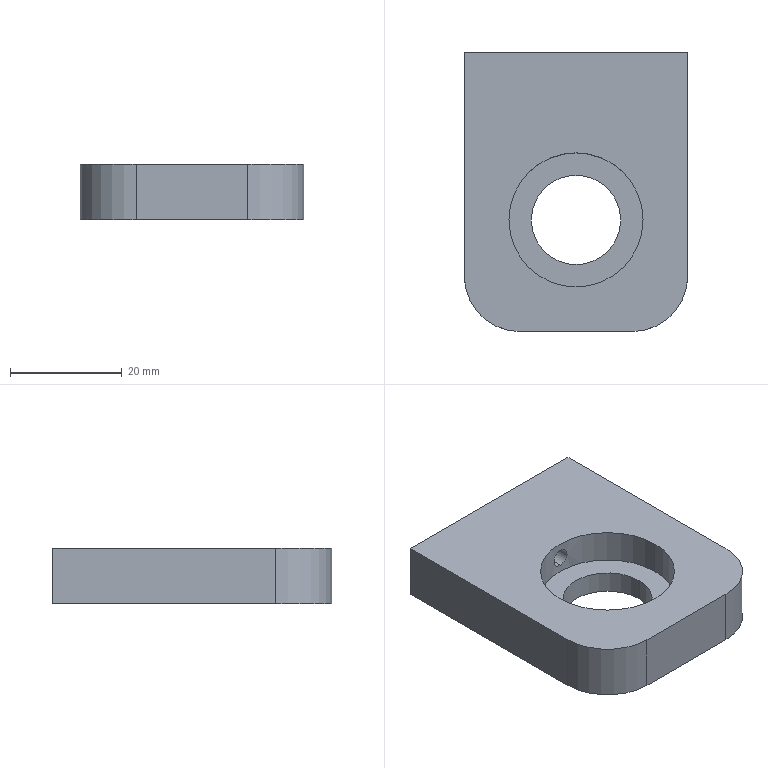Part | SolidWorks | features HoleWzd 2, ICE 2, Extrusion 1, Fillet 1 | 1 solid | 23 faces | box 40 x 50 x 10 mm | volume 15721 mm3 | cylinder 12 | plane 7 | cone 4 | commonest cylinder face diameters 3.3 x6 16 x2 20 x2 24 x2
STEP:
#1=CARTESIAN_POINT('',(0.,7.,5.35));
#2=VERTEX_POINT('',#1);
#3=CARTESIAN_POINT('',(0.,7.,8.65));
#4=VERTEX_POINT('',#3);
#5=CARTESIAN_POINT('',(0.,7.,5.35));
#6=CARTESIAN_POINT('',(-0.2155,7.,5.35));
#7=CARTESIAN_POINT('',(-0.4328,6.994,5.393));
#8=CARTESIAN_POINT('',(-0.8299,6.973,5.558));
#9=CARTESIAN_POINT('',(-1.014,6.958,5.681));
#10=CARTESIAN_POINT('',(-1.242,6.936,5.908));
#11=CARTESIAN_POINT('',(-1.312,6.928,5.993));
#12=CARTESIAN_POINT('',(-1.431,6.914,6.172));
#13=CARTESIAN_POINT('',(-1.482,6.908,6.267));
#14=CARTESIAN_POINT('',(-1.565,6.898,6.467));
#15=CARTESIAN_POINT('',(-1.597,6.893,6.571));
#16=CARTESIAN_POINT('',(-1.639,6.888,6.782));
#17=CARTESIAN_POINT('',(-1.65,6.886,6.89));
#18=CARTESIAN_POINT('',(-1.65,6.886,7.108));
#19=CARTESIAN_POINT('',(-1.639,6.888,7.215));
#20=CARTESIAN_POINT('',(-1.598,6.893,7.426));
#21=CARTESIAN_POINT('',(-1.566,6.897,7.531));
#22=CARTESIAN_POINT('',(-1.483,6.908,7.731));
#23=CARTESIAN_POINT('',(-1.433,6.914,7.826));
#24=CARTESIAN_POINT('',(-1.313,6.928,8.005));
#25=CARTESIAN_POINT('',(-1.243,6.936,8.09));
#26=CARTESIAN_POINT('',(-1.016,6.958,8.318));
#27=CARTESIAN_POINT('',(-0.8319,6.973,8.441));
#28=CARTESIAN_POINT('',(-0.4351,6.994,8.606));
#29=CARTESIAN_POINT('',(-0.2183,7.,8.65));
#30=CARTESIAN_POINT('',(0.,7.,8.65));
#31=B_SPLINE_CURVE_WITH_KNOTS('',3,(#5,#6,#7,#8,#9,#10,#11,#12,#13,#14,#15,#16,#17,#18,#19,#20,#21,#22,#23,#24,#25,#26,#27,#28,#29,#30),.UNSPECIFIED.,.F.,.F.,(4,2,2,2,2,2,2,2,2,2,2,2,4),(0.005165,0.00581,0.006456,0.006778,0.007101,0.007424,0.007747,0.008069,0.008392,0.008715,0.009037,0.009683,0.01033),.UNSPECIFIED.);
#32=EDGE_CURVE('',#2,#4,#31,.T.);
#33=ORIENTED_EDGE('',*,*,#32,.F.);
#34=CARTESIAN_POINT('',(0.,25.,5.35));
#35=VERTEX_POINT('',#34);
#36=CARTESIAN_POINT('',(0.,25.,5.35));
#37=DIRECTION('',(0.,1.,0.));
#38=VECTOR('',#37,1000.);
#39=LINE('',#36,#38);
#40=EDGE_CURVE('',#2,#35,#39,.T.);
#41=ORIENTED_EDGE('',*,*,#40,.T.);
#42=CARTESIAN_POINT('',(0.,25.,8.65));
#43=VERTEX_POINT('',#42);
#44=CARTESIAN_POINT('',(0.,25.,7.));
#45=DIRECTION('',(0.,1.,0.));
#46=DIRECTION('',(0.,0.,1.));
#47=AXIS2_PLACEMENT_3D('',#44,#45,#46);
#48=CIRCLE('',#47,1.65);
#49=EDGE_CURVE('',#35,#43,#48,.T.);
#50=ORIENTED_EDGE('',*,*,#49,.T.);
#51=CARTESIAN_POINT('',(0.,25.,8.65));
#52=DIRECTION('',(0.,1.,0.));
#53=VECTOR('',#52,1000.);
#54=LINE('',#51,#53);
#55=EDGE_CURVE('',#4,#43,#54,.T.);
#56=ORIENTED_EDGE('',*,*,#55,.F.);
#57=EDGE_LOOP('',(#33,#41,#50,#56));
#58=FACE_OUTER_BOUND('',#57,.T.);
#59=CARTESIAN_POINT('',(0.,25.,7.));
#60=DIRECTION('',(0.,1.,0.));
#61=DIRECTION('',(0.,0.,1.));
#62=AXIS2_PLACEMENT_3D('',#59,#60,#61);
#63=CYLINDRICAL_SURFACE('',#62,1.65);
#64=ADVANCED_FACE('',(#58),#63,.F.);
#65=CARTESIAN_POINT('',(-15.,15.,3.35));
#66=VERTEX_POINT('',#65);
#67=CARTESIAN_POINT('',(-15.,15.,6.65));
#68=VERTEX_POINT('',#67);
#69=CARTESIAN_POINT('',(-15.,15.,5.));
#70=DIRECTION('',(0.,1.,0.));
#71=DIRECTION('',(0.,0.,1.));
#72=AXIS2_PLACEMENT_3D('',#69,#70,#71);
#73=CIRCLE('',#72,1.65);
#74=EDGE_CURVE('',#66,#68,#73,.T.);
#75=ORIENTED_EDGE('',*,*,#74,.F.);
#76=CARTESIAN_POINT('',(-15.,25.,3.35));
#77=VERTEX_POINT('',#76);
#78=CARTESIAN_POINT('',(-15.,25.,3.35));
#79=DIRECTION('',(0.,1.,0.));
#80=VECTOR('',#79,1000.);
#81=LINE('',#78,#80);
#82=EDGE_CURVE('',#66,#77,#81,.T.);
#83=ORIENTED_EDGE('',*,*,#82,.T.);
#84=CARTESIAN_POINT('',(-15.,25.,6.65));
#85=VERTEX_POINT('',#84);
#86=CARTESIAN_POINT('',(-15.,25.,5.));
#87=DIRECTION('',(0.,1.,0.));
#88=DIRECTION('',(0.,0.,1.));
#89=AXIS2_PLACEMENT_3D('',#86,#87,#88);
#90=CIRCLE('',#89,1.65);
#91=EDGE_CURVE('',#77,#85,#90,.T.);
#92=ORIENTED_EDGE('',*,*,#91,.T.);
#93=CARTESIAN_POINT('',(-15.,25.,6.65));
#94=DIRECTION('',(0.,1.,0.));
#95=VECTOR('',#94,1000.);
#96=LINE('',#93,#95);
#97=EDGE_CURVE('',#68,#85,#96,.T.);
#98=ORIENTED_EDGE('',*,*,#97,.F.);
#99=EDGE_LOOP('',(#75,#83,#92,#98));
#100=FACE_OUTER_BOUND('',#99,.T.);
#101=CARTESIAN_POINT('',(-15.,25.,5.));
#102=DIRECTION('',(0.,1.,0.));
#103=DIRECTION('',(0.,0.,1.));
#104=AXIS2_PLACEMENT_3D('',#101,#102,#103);
#105=CYLINDRICAL_SURFACE('',#104,1.65);
#106=ADVANCED_FACE('',(#100),#105,.F.);
#107=CARTESIAN_POINT('',(-15.,14.009,5.));
#108=VERTEX_POINT('',#107);
#109=CARTESIAN_POINT('',(-15.,15.,6.65));
#110=DIRECTION('',(0.,0.515,0.8572));
#111=VECTOR('',#110,1000.);
#112=LINE('',#109,#111);
#113=EDGE_CURVE('',#108,#68,#112,.T.);
#114=ORIENTED_EDGE('',*,*,#113,.F.);
#115=CARTESIAN_POINT('',(-15.,15.,3.35));
#116=DIRECTION('',(0.,0.515,-0.8572));
#117=VECTOR('',#116,1000.);
#118=LINE('',#115,#117);
#119=EDGE_CURVE('',#108,#66,#118,.T.);
#120=ORIENTED_EDGE('',*,*,#119,.T.);
#121=ORIENTED_EDGE('',*,*,#74,.T.);
#122=EDGE_LOOP('',(#114,#120,#121));
#123=FACE_OUTER_BOUND('',#122,.T.);
#124=CARTESIAN_POINT('',(-15.,15.,5.));
#125=DIRECTION('',(0.,1.,0.));
#126=DIRECTION('',(0.,0.,1.));
#127=AXIS2_PLACEMENT_3D('',#124,#125,#126);
#128=CONICAL_SURFACE('',#127,1.65,1.03);
#129=ADVANCED_FACE('',(#123),#128,.F.);
#130=CARTESIAN_POINT('',(15.,15.,3.35));
#131=VERTEX_POINT('',#130);
#132=CARTESIAN_POINT('',(15.,15.,6.65));
#133=VERTEX_POINT('',#132);
#134=CARTESIAN_POINT('',(15.,15.,5.));
#135=DIRECTION('',(0.,1.,0.));
#136=DIRECTION('',(0.,0.,1.));
#137=AXIS2_PLACEMENT_3D('',#134,#135,#136);
#138=CIRCLE('',#137,1.65);
#139=EDGE_CURVE('',#131,#133,#138,.T.);
#140=ORIENTED_EDGE('',*,*,#139,.F.);
#141=CARTESIAN_POINT('',(15.,25.,3.35));
#142=VERTEX_POINT('',#141);
#143=CARTESIAN_POINT('',(15.,25.,3.35));
#144=DIRECTION('',(0.,1.,0.));
#145=VECTOR('',#144,1000.);
#146=LINE('',#143,#145);
#147=EDGE_CURVE('',#131,#142,#146,.T.);
#148=ORIENTED_EDGE('',*,*,#147,.T.);
#149=CARTESIAN_POINT('',(15.,25.,6.65));
#150=VERTEX_POINT('',#149);
#151=CARTESIAN_POINT('',(15.,25.,5.));
#152=DIRECTION('',(0.,1.,0.));
#153=DIRECTION('',(0.,0.,1.));
#154=AXIS2_PLACEMENT_3D('',#151,#152,#153);
#155=CIRCLE('',#154,1.65);
#156=EDGE_CURVE('',#142,#150,#155,.T.);
#157=ORIENTED_EDGE('',*,*,#156,.T.);
#158=CARTESIAN_POINT('',(15.,25.,6.65));
#159=DIRECTION('',(0.,1.,0.));
#160=VECTOR('',#159,1000.);
#161=LINE('',#158,#160);
#162=EDGE_CURVE('',#133,#150,#161,.T.);
#163=ORIENTED_EDGE('',*,*,#162,.F.);
#164=EDGE_LOOP('',(#140,#148,#157,#163));
#165=FACE_OUTER_BOUND('',#164,.T.);
#166=CARTESIAN_POINT('',(15.,25.,5.));
#167=DIRECTION('',(0.,1.,0.));
#168=DIRECTION('',(0.,0.,1.));
#169=AXIS2_PLACEMENT_3D('',#166,#167,#168);
#170=CYLINDRICAL_SURFACE('',#169,1.65);
#171=ADVANCED_FACE('',(#165),#170,.F.);
#172=CARTESIAN_POINT('',(15.,14.009,5.));
#173=VERTEX_POINT('',#172);
#174=CARTESIAN_POINT('',(15.,15.,6.65));
#175=DIRECTION('',(0.,0.515,0.8572));
#176=VECTOR('',#175,1000.);
#177=LINE('',#174,#176);
#178=EDGE_CURVE('',#173,#133,#177,.T.);
#179=ORIENTED_EDGE('',*,*,#178,.F.);
#180=CARTESIAN_POINT('',(15.,15.,3.35));
#181=DIRECTION('',(0.,0.515,-0.8572));
#182=VECTOR('',#181,1000.);
#183=LINE('',#180,#182);
#184=EDGE_CURVE('',#173,#131,#183,.T.);
#185=ORIENTED_EDGE('',*,*,#184,.T.);
#186=ORIENTED_EDGE('',*,*,#139,.T.);
#187=EDGE_LOOP('',(#179,#185,#186));
#188=FACE_OUTER_BOUND('',#187,.T.);
#189=CARTESIAN_POINT('',(15.,15.,5.));
#190=DIRECTION('',(0.,1.,0.));
#191=DIRECTION('',(0.,0.,1.));
#192=AXIS2_PLACEMENT_3D('',#189,#190,#191);
#193=CONICAL_SURFACE('',#192,1.65,1.03);
#194=ADVANCED_FACE('',(#188),#193,.F.);
#195=CARTESIAN_POINT('',(-8.,-5.,0.));
#196=VERTEX_POINT('',#195);
#197=CARTESIAN_POINT('',(8.,-5.,0.));
#198=VERTEX_POINT('',#197);
#199=CARTESIAN_POINT('',(0.,-5.,0.));
#200=DIRECTION('',(0.,0.,1.));
#201=DIRECTION('',(1.,0.,0.));
#202=AXIS2_PLACEMENT_3D('',#199,#200,#201);
#203=CIRCLE('',#202,8.);
#204=EDGE_CURVE('',#196,#198,#203,.T.);
#205=ORIENTED_EDGE('',*,*,#204,.F.);
#206=CARTESIAN_POINT('',(-8.,-5.,4.));
#207=VERTEX_POINT('',#206);
#208=CARTESIAN_POINT('',(-8.,-5.,0.));
#209=DIRECTION('',(0.,0.,1.));
#210=VECTOR('',#209,1000.);
#211=LINE('',#208,#210);
#212=EDGE_CURVE('',#196,#207,#211,.T.);
#213=ORIENTED_EDGE('',*,*,#212,.T.);
#214=CARTESIAN_POINT('',(8.,-5.,4.));
#215=VERTEX_POINT('',#214);
#216=CARTESIAN_POINT('',(0.,-5.,4.));
#217=DIRECTION('',(0.,0.,1.));
#218=DIRECTION('',(1.,0.,0.));
#219=AXIS2_PLACEMENT_3D('',#216,#217,#218);
#220=CIRCLE('',#219,8.);
#221=EDGE_CURVE('',#207,#215,#220,.T.);
#222=ORIENTED_EDGE('',*,*,#221,.T.);
#223=CARTESIAN_POINT('',(8.,-5.,0.));
#224=DIRECTION('',(0.,0.,1.));
#225=VECTOR('',#224,1000.);
#226=LINE('',#223,#225);
#227=EDGE_CURVE('',#198,#215,#226,.T.);
#228=ORIENTED_EDGE('',*,*,#227,.F.);
#229=EDGE_LOOP('',(#205,#213,#222,#228));
#230=FACE_OUTER_BOUND('',#229,.T.);
#231=CARTESIAN_POINT('',(0.,-5.,0.));
#232=DIRECTION('',(0.,0.,1.));
#233=DIRECTION('',(1.,0.,0.));
#234=AXIS2_PLACEMENT_3D('',#231,#232,#233);
#235=CYLINDRICAL_SURFACE('',#234,8.);
#236=ADVANCED_FACE('',(#230),#235,.F.);
#237=CARTESIAN_POINT('',(-12.,-5.,4.));
#238=VERTEX_POINT('',#237);
#239=CARTESIAN_POINT('',(12.,-5.,4.));
#240=VERTEX_POINT('',#239);
#241=CARTESIAN_POINT('',(0.,-5.,4.));
#242=DIRECTION('',(0.,0.,1.));
#243=DIRECTION('',(1.,0.,0.));
#244=AXIS2_PLACEMENT_3D('',#241,#242,#243);
#245=CIRCLE('',#244,12.);
#246=EDGE_CURVE('',#238,#240,#245,.T.);
#247=ORIENTED_EDGE('',*,*,#246,.F.);
#248=CARTESIAN_POINT('',(-12.,-5.,10.));
#249=VERTEX_POINT('',#248);
#250=CARTESIAN_POINT('',(-12.,-5.,4.));
#251=DIRECTION('',(0.,0.,1.));
#252=VECTOR('',#251,1000.);
#253=LINE('',#250,#252);
#254=EDGE_CURVE('',#238,#249,#253,.T.);
#255=ORIENTED_EDGE('',*,*,#254,.T.);
#256=CARTESIAN_POINT('',(12.,-5.,10.));
#257=VERTEX_POINT('',#256);
#258=CARTESIAN_POINT('',(0.,-5.,10.));
#259=DIRECTION('',(0.,0.,1.));
#260=DIRECTION('',(1.,0.,0.));
#261=AXIS2_PLACEMENT_3D('',#258,#259,#260);
#262=CIRCLE('',#261,12.);
#263=EDGE_CURVE('',#249,#257,#262,.T.);
#264=ORIENTED_EDGE('',*,*,#263,.T.);
#265=CARTESIAN_POINT('',(12.,-5.,4.));
#266=DIRECTION('',(0.,0.,1.));
#267=VECTOR('',#266,1000.);
#268=LINE('',#265,#267);
#269=EDGE_CURVE('',#240,#257,#268,.T.);
#270=ORIENTED_EDGE('',*,*,#269,.F.);
#271=EDGE_LOOP('',(#247,#255,#264,#270));
#272=FACE_OUTER_BOUND('',#271,.T.);
#273=CARTESIAN_POINT('',(0.,-5.,4.));
#274=DIRECTION('',(0.,0.,1.));
#275=DIRECTION('',(1.,0.,0.));
#276=AXIS2_PLACEMENT_3D('',#273,#274,#275);
#277=CYLINDRICAL_SURFACE('',#276,12.);
#278=ADVANCED_FACE('',(#272),#277,.F.);
#279=CARTESIAN_POINT('',(-20.,25.,0.));
#280=VERTEX_POINT('',#279);
#281=CARTESIAN_POINT('',(-20.,-15.,0.));
#282=VERTEX_POINT('',#281);
#283=CARTESIAN_POINT('',(-20.,25.,0.));
#284=DIRECTION('',(0.,-1.,0.));
#285=VECTOR('',#284,1000.);
#286=LINE('',#283,#285);
#287=EDGE_CURVE('',#280,#282,#286,.T.);
#288=ORIENTED_EDGE('',*,*,#287,.T.);
#289=CARTESIAN_POINT('',(-20.,-15.,10.));
#290=VERTEX_POINT('',#289);
#291=CARTESIAN_POINT('',(-20.,-15.,10.));
#292=DIRECTION('',(0.,0.,1.));
#293=VECTOR('',#292,1000.);
#294=LINE('',#291,#293);
#295=EDGE_CURVE('',#282,#290,#294,.T.);
#296=ORIENTED_EDGE('',*,*,#295,.T.);
#297=CARTESIAN_POINT('',(-20.,25.,10.));
#298=VERTEX_POINT('',#297);
#299=CARTESIAN_POINT('',(-20.,25.,10.));
#300=DIRECTION('',(0.,-1.,0.));
#301=VECTOR('',#300,1000.);
#302=LINE('',#299,#301);
#303=EDGE_CURVE('',#298,#290,#302,.T.);
#304=ORIENTED_EDGE('',*,*,#303,.F.);
#305=CARTESIAN_POINT('',(-20.,25.,10.));
#306=DIRECTION('',(0.,0.,-1.));
#307=VECTOR('',#306,1000.);
#308=LINE('',#305,#307);
#309=EDGE_CURVE('',#298,#280,#308,.T.);
#310=ORIENTED_EDGE('',*,*,#309,.T.);
#311=EDGE_LOOP('',(#288,#296,#304,#310));
#312=FACE_OUTER_BOUND('',#311,.T.);
#313=CARTESIAN_POINT('',(-20.,25.,10.));
#314=DIRECTION('',(1.,0.,0.));
#315=DIRECTION('',(0.,1.,0.));
#316=AXIS2_PLACEMENT_3D('',#313,#314,#315);
#317=PLANE('',#316);
#318=ADVANCED_FACE('',(#312),#317,.F.);
#319=CARTESIAN_POINT('',(-10.,-25.,10.));
#320=VERTEX_POINT('',#319);
#321=CARTESIAN_POINT('',(10.,-25.,10.));
#322=VERTEX_POINT('',#321);
#323=CARTESIAN_POINT('',(20.,-25.,10.));
#324=DIRECTION('',(1.,0.,0.));
#325=VECTOR('',#324,1000.);
#326=LINE('',#323,#325);
#327=EDGE_CURVE('',#320,#322,#326,.T.);
#328=ORIENTED_EDGE('',*,*,#327,.F.);
#329=CARTESIAN_POINT('',(-10.,-25.,0.));
#330=VERTEX_POINT('',#329);
#331=CARTESIAN_POINT('',(-10.,-25.,10.));
#332=DIRECTION('',(0.,0.,-1.));
#333=VECTOR('',#332,1000.);
#334=LINE('',#331,#333);
#335=EDGE_CURVE('',#320,#330,#334,.T.);
#336=ORIENTED_EDGE('',*,*,#335,.T.);
#337=CARTESIAN_POINT('',(10.,-25.,0.));
#338=VERTEX_POINT('',#337);
#339=CARTESIAN_POINT('',(20.,-25.,0.));
#340=DIRECTION('',(1.,0.,0.));
#341=VECTOR('',#340,1000.);
#342=LINE('',#339,#341);
#343=EDGE_CURVE('',#330,#338,#342,.T.);
#344=ORIENTED_EDGE('',*,*,#343,.T.);
#345=CARTESIAN_POINT('',(10.,-25.,10.));
#346=DIRECTION('',(0.,0.,1.));
#347=VECTOR('',#346,1000.);
#348=LINE('',#345,#347);
#349=EDGE_CURVE('',#338,#322,#348,.T.);
#350=ORIENTED_EDGE('',*,*,#349,.T.);
#351=EDGE_LOOP('',(#328,#336,#344,#350));
#352=FACE_OUTER_BOUND('',#351,.T.);
#353=CARTESIAN_POINT('',(20.,-25.,10.));
#354=DIRECTION('',(0.,1.,0.));
#355=DIRECTION('',(-1.,0.,0.));
#356=AXIS2_PLACEMENT_3D('',#353,#354,#355);
#357=PLANE('',#356);
#358=ADVANCED_FACE('',(#352),#357,.F.);
#359=CARTESIAN_POINT('',(20.,-15.,10.));
#360=VERTEX_POINT('',#359);
#361=CARTESIAN_POINT('',(20.,25.,10.));
#362=VERTEX_POINT('',#361);
#363=CARTESIAN_POINT('',(20.,25.,10.));
#364=DIRECTION('',(0.,1.,0.));
#365=VECTOR('',#364,1000.);
#366=LINE('',#363,#365);
#367=EDGE_CURVE('',#360,#362,#366,.T.);
#368=ORIENTED_EDGE('',*,*,#367,.F.);
#369=CARTESIAN_POINT('',(20.,-15.,0.));
#370=VERTEX_POINT('',#369);
#371=CARTESIAN_POINT('',(20.,-15.,10.));
#372=DIRECTION('',(0.,0.,-1.));
#373=VECTOR('',#372,1000.);
#374=LINE('',#371,#373);
#375=EDGE_CURVE('',#360,#370,#374,.T.);
#376=ORIENTED_EDGE('',*,*,#375,.T.);
#377=CARTESIAN_POINT('',(20.,25.,0.));
#378=VERTEX_POINT('',#377);
#379=CARTESIAN_POINT('',(20.,25.,0.));
#380=DIRECTION('',(0.,1.,0.));
#381=VECTOR('',#380,1000.);
#382=LINE('',#379,#381);
#383=EDGE_CURVE('',#370,#378,#382,.T.);
#384=ORIENTED_EDGE('',*,*,#383,.T.);
#385=CARTESIAN_POINT('',(20.,25.,10.));
#386=DIRECTION('',(0.,0.,-1.));
#387=VECTOR('',#386,1000.);
#388=LINE('',#385,#387);
#389=EDGE_CURVE('',#362,#378,#388,.T.);
#390=ORIENTED_EDGE('',*,*,#389,.F.);
#391=EDGE_LOOP('',(#368,#376,#384,#390));
#392=FACE_OUTER_BOUND('',#391,.T.);
#393=CARTESIAN_POINT('',(20.,25.,10.));
#394=DIRECTION('',(-1.,0.,0.));
#395=DIRECTION('',(0.,-1.,0.));
#396=AXIS2_PLACEMENT_3D('',#393,#394,#395);
#397=PLANE('',#396);
#398=ADVANCED_FACE('',(#392),#397,.F.);
#399=CARTESIAN_POINT('',(0.,25.,7.));
#400=DIRECTION('',(0.,1.,0.));
#401=DIRECTION('',(0.,0.,1.));
#402=AXIS2_PLACEMENT_3D('',#399,#400,#401);
#403=CIRCLE('',#402,1.65);
#404=EDGE_CURVE('',#43,#35,#403,.T.);
#405=ORIENTED_EDGE('',*,*,#404,.F.);
#406=ORIENTED_EDGE('',*,*,#49,.F.);
#407=EDGE_LOOP('',(#405,#406));
#408=FACE_BOUND('',#407,.T.);
#409=CARTESIAN_POINT('',(-15.,25.,5.));
#410=DIRECTION('',(0.,1.,0.));
#411=DIRECTION('',(0.,0.,1.));
#412=AXIS2_PLACEMENT_3D('',#409,#410,#411);
#413=CIRCLE('',#412,1.65);
#414=EDGE_CURVE('',#85,#77,#413,.T.);
#415=ORIENTED_EDGE('',*,*,#414,.F.);
#416=ORIENTED_EDGE('',*,*,#91,.F.);
#417=EDGE_LOOP('',(#415,#416));
#418=FACE_BOUND('',#417,.T.);
#419=CARTESIAN_POINT('',(15.,25.,5.));
#420=DIRECTION('',(0.,1.,0.));
#421=DIRECTION('',(0.,0.,1.));
#422=AXIS2_PLACEMENT_3D('',#419,#420,#421);
#423=CIRCLE('',#422,1.65);
#424=EDGE_CURVE('',#150,#142,#423,.T.);
#425=ORIENTED_EDGE('',*,*,#424,.F.);
#426=ORIENTED_EDGE('',*,*,#156,.F.);
#427=EDGE_LOOP('',(#425,#426));
#428=FACE_BOUND('',#427,.T.);
#429=CARTESIAN_POINT('',(20.,25.,0.));
#430=DIRECTION('',(-1.,0.,0.));
#431=VECTOR('',#430,1000.);
#432=LINE('',#429,#431);
#433=EDGE_CURVE('',#378,#280,#432,.T.);
#434=ORIENTED_EDGE('',*,*,#433,.T.);
#435=ORIENTED_EDGE('',*,*,#309,.F.);
#436=CARTESIAN_POINT('',(20.,25.,10.));
#437=DIRECTION('',(-1.,0.,0.));
#438=VECTOR('',#437,1000.);
#439=LINE('',#436,#438);
#440=EDGE_CURVE('',#362,#298,#439,.T.);
#441=ORIENTED_EDGE('',*,*,#440,.F.);
#442=ORIENTED_EDGE('',*,*,#389,.T.);
#443=EDGE_LOOP('',(#434,#435,#441,#442));
#444=FACE_OUTER_BOUND('',#443,.T.);
#445=CARTESIAN_POINT('',(20.,25.,10.));
#446=DIRECTION('',(0.,-1.,0.));
#447=DIRECTION('',(1.,0.,0.));
#448=AXIS2_PLACEMENT_3D('',#445,#446,#447);
#449=PLANE('',#448);
#450=ADVANCED_FACE('',(#408,#418,#428,#444),#449,.F.);
#451=CARTESIAN_POINT('',(0.,-5.,10.));
#452=DIRECTION('',(0.,0.,1.));
#453=DIRECTION('',(1.,0.,0.));
#454=AXIS2_PLACEMENT_3D('',#451,#452,#453);
#455=CIRCLE('',#454,12.);
#456=EDGE_CURVE('',#257,#249,#455,.T.);
#457=ORIENTED_EDGE('',*,*,#456,.F.);
#458=ORIENTED_EDGE('',*,*,#263,.F.);
#459=EDGE_LOOP('',(#457,#458));
#460=FACE_BOUND('',#459,.T.);
#461=ORIENTED_EDGE('',*,*,#303,.T.);
#462=CARTESIAN_POINT('',(-10.,-15.,10.));
#463=DIRECTION('',(0.,0.,1.));
#464=DIRECTION('',(-1.,0.,0.));
#465=AXIS2_PLACEMENT_3D('',#462,#463,#464);
#466=CIRCLE('',#465,10.);
#467=EDGE_CURVE('',#290,#320,#466,.T.);
#468=ORIENTED_EDGE('',*,*,#467,.T.);
#469=ORIENTED_EDGE('',*,*,#327,.T.);
#470=CARTESIAN_POINT('',(10.,-15.,10.));
#471=DIRECTION('',(0.,0.,1.));
#472=DIRECTION('',(-1.,0.,0.));
#473=AXIS2_PLACEMENT_3D('',#470,#471,#472);
#474=CIRCLE('',#473,10.);
#475=EDGE_CURVE('',#322,#360,#474,.T.);
#476=ORIENTED_EDGE('',*,*,#475,.T.);
#477=ORIENTED_EDGE('',*,*,#367,.T.);
#478=ORIENTED_EDGE('',*,*,#440,.T.);
#479=EDGE_LOOP('',(#461,#468,#469,#476,#477,#478));
#480=FACE_OUTER_BOUND('',#479,.T.);
#481=CARTESIAN_POINT('',(0.,0.,10.));
#482=DIRECTION('',(0.,0.,-1.));
#483=DIRECTION('',(-1.,0.,0.));
#484=AXIS2_PLACEMENT_3D('',#481,#482,#483);
#485=PLANE('',#484);
#486=ADVANCED_FACE('',(#460,#480),#485,.F.);
#487=CARTESIAN_POINT('',(0.,-5.,0.));
#488=DIRECTION('',(0.,0.,1.));
#489=DIRECTION('',(1.,0.,0.));
#490=AXIS2_PLACEMENT_3D('',#487,#488,#489);
#491=CIRCLE('',#490,8.);
#492=EDGE_CURVE('',#198,#196,#491,.T.);
#493=ORIENTED_EDGE('',*,*,#492,.T.);
#494=ORIENTED_EDGE('',*,*,#204,.T.);
#495=EDGE_LOOP('',(#493,#494));
#496=FACE_BOUND('',#495,.T.);
#497=ORIENTED_EDGE('',*,*,#343,.F.);
#498=CARTESIAN_POINT('',(-10.,-15.,0.));
#499=DIRECTION('',(0.,0.,-1.));
#500=DIRECTION('',(-1.,0.,0.));
#501=AXIS2_PLACEMENT_3D('',#498,#499,#500);
#502=CIRCLE('',#501,10.);
#503=EDGE_CURVE('',#330,#282,#502,.T.);
#504=ORIENTED_EDGE('',*,*,#503,.T.);
#505=ORIENTED_EDGE('',*,*,#287,.F.);
#506=ORIENTED_EDGE('',*,*,#433,.F.);
#507=ORIENTED_EDGE('',*,*,#383,.F.);
#508=CARTESIAN_POINT('',(10.,-15.,0.));
#509=DIRECTION('',(0.,0.,-1.));
#510=DIRECTION('',(-1.,0.,0.));
#511=AXIS2_PLACEMENT_3D('',#508,#509,#510);
#512=CIRCLE('',#511,10.);
#513=EDGE_CURVE('',#370,#338,#512,.T.);
#514=ORIENTED_EDGE('',*,*,#513,.T.);
#515=EDGE_LOOP('',(#497,#504,#505,#506,#507,#514));
#516=FACE_OUTER_BOUND('',#515,.T.);
#517=CARTESIAN_POINT('',(0.,0.,0.));
#518=DIRECTION('',(0.,0.,-1.));
#519=DIRECTION('',(-1.,0.,0.));
#520=AXIS2_PLACEMENT_3D('',#517,#518,#519);
#521=PLANE('',#520);
#522=ADVANCED_FACE('',(#496,#516),#521,.T.);
#523=ORIENTED_EDGE('',*,*,#254,.F.);
#524=CARTESIAN_POINT('',(0.,-5.,4.));
#525=DIRECTION('',(0.,0.,1.));
#526=DIRECTION('',(1.,0.,0.));
#527=AXIS2_PLACEMENT_3D('',#524,#525,#526);
#528=CIRCLE('',#527,12.);
#529=EDGE_CURVE('',#240,#238,#528,.T.);
#530=ORIENTED_EDGE('',*,*,#529,.F.);
#531=ORIENTED_EDGE('',*,*,#269,.T.);
#532=ORIENTED_EDGE('',*,*,#456,.T.);
#533=EDGE_LOOP('',(#523,#530,#531,#532));
#534=FACE_OUTER_BOUND('',#533,.T.);
#535=CARTESIAN_POINT('',(0.,7.,8.65));
#536=CARTESIAN_POINT('',(0.1092,7.,8.65));
#537=CARTESIAN_POINT('',(0.2165,6.999,8.639));
#538=CARTESIAN_POINT('',(0.4275,6.993,8.597));
#539=CARTESIAN_POINT('',(0.5324,6.989,8.565));
#540=CARTESIAN_POINT('',(0.7322,6.978,8.483));
#541=CARTESIAN_POINT('',(0.8269,6.972,8.432));
#542=CARTESIAN_POINT('',(1.006,6.958,8.312));
#543=CARTESIAN_POINT('',(1.091,6.951,8.243));
#544=CARTESIAN_POINT('',(1.319,6.928,8.014));
#545=CARTESIAN_POINT('',(1.442,6.913,7.831));
#546=CARTESIAN_POINT('',(1.606,6.892,7.433));
#547=CARTESIAN_POINT('',(1.65,6.886,7.216));
#548=CARTESIAN_POINT('',(1.65,6.886,6.893));
#549=CARTESIAN_POINT('',(1.639,6.888,6.783));
#550=CARTESIAN_POINT('',(1.597,6.893,6.572));
#551=CARTESIAN_POINT('',(1.566,6.897,6.469));
#552=CARTESIAN_POINT('',(1.483,6.908,6.269));
#553=CARTESIAN_POINT('',(1.431,6.914,6.172));
#554=CARTESIAN_POINT('',(1.312,6.928,5.994));
#555=CARTESIAN_POINT('',(1.244,6.936,5.91));
#556=CARTESIAN_POINT('',(1.09,6.951,5.756));
#557=CARTESIAN_POINT('',(1.007,6.958,5.688));
#558=CARTESIAN_POINT('',(0.8281,6.972,5.569));
#559=CARTESIAN_POINT('',(0.7315,6.978,5.517));
#560=CARTESIAN_POINT('',(0.5318,6.989,5.434));
#561=CARTESIAN_POINT('',(0.4289,6.993,5.403));
#562=CARTESIAN_POINT('',(0.2172,6.999,5.361));
#563=CARTESIAN_POINT('',(0.1078,7.,5.35));
#564=CARTESIAN_POINT('',(0.,7.,5.35));
#565=B_SPLINE_CURVE_WITH_KNOTS('',3,(#535,#536,#537,#538,#539,#540,#541,#542,#543,#544,#545,#546,#547,#548,#549,#550,#551,#552,#553,#554,#555,#556,#557,#558,#559,#560,#561,#562,#563,#564),.UNSPECIFIED.,.F.,.F.,(4,2,2,2,2,2,2,2,2,2,2,2,2,2,4),(0.,0.0003228,0.0006456,0.0009684,0.001291,0.001937,0.002582,0.002905,0.003228,0.003551,0.003874,0.004196,0.004519,0.004842,0.005165),.UNSPECIFIED.);
#566=EDGE_CURVE('',#4,#2,#565,.T.);
#567=ORIENTED_EDGE('',*,*,#566,.T.);
#568=ORIENTED_EDGE('',*,*,#32,.T.);
#569=EDGE_LOOP('',(#567,#568));
#570=FACE_BOUND('',#569,.T.);
#571=CARTESIAN_POINT('',(0.,-5.,4.));
#572=DIRECTION('',(0.,0.,1.));
#573=DIRECTION('',(1.,0.,0.));
#574=AXIS2_PLACEMENT_3D('',#571,#572,#573);
#575=CYLINDRICAL_SURFACE('',#574,12.);
#576=ADVANCED_FACE('',(#534,#570),#575,.F.);
#577=CARTESIAN_POINT('',(0.,-5.,4.));
#578=DIRECTION('',(0.,0.,1.));
#579=DIRECTION('',(1.,0.,0.));
#580=AXIS2_PLACEMENT_3D('',#577,#578,#579);
#581=CIRCLE('',#580,8.);
#582=EDGE_CURVE('',#215,#207,#581,.T.);
#583=ORIENTED_EDGE('',*,*,#582,.F.);
#584=ORIENTED_EDGE('',*,*,#221,.F.);
#585=EDGE_LOOP('',(#583,#584));
#586=FACE_BOUND('',#585,.T.);
#587=ORIENTED_EDGE('',*,*,#529,.T.);
#588=ORIENTED_EDGE('',*,*,#246,.T.);
#589=EDGE_LOOP('',(#587,#588));
#590=FACE_OUTER_BOUND('',#589,.T.);
#591=CARTESIAN_POINT('',(0.,-5.,4.));
#592=DIRECTION('',(0.,0.,1.));
#593=DIRECTION('',(1.,0.,0.));
#594=AXIS2_PLACEMENT_3D('',#591,#592,#593);
#595=PLANE('',#594);
#596=ADVANCED_FACE('',(#586,#590),#595,.T.);
#597=ORIENTED_EDGE('',*,*,#212,.F.);
#598=ORIENTED_EDGE('',*,*,#492,.F.);
#599=ORIENTED_EDGE('',*,*,#227,.T.);
#600=ORIENTED_EDGE('',*,*,#582,.T.);
#601=EDGE_LOOP('',(#597,#598,#599,#600));
#602=FACE_OUTER_BOUND('',#601,.T.);
#603=CARTESIAN_POINT('',(0.,-5.,0.));
#604=DIRECTION('',(0.,0.,1.));
#605=DIRECTION('',(1.,0.,0.));
#606=AXIS2_PLACEMENT_3D('',#603,#604,#605);
#607=CYLINDRICAL_SURFACE('',#606,8.);
#608=ADVANCED_FACE('',(#602),#607,.F.);
#609=ORIENTED_EDGE('',*,*,#184,.F.);
#610=ORIENTED_EDGE('',*,*,#178,.T.);
#611=CARTESIAN_POINT('',(15.,15.,5.));
#612=DIRECTION('',(0.,1.,0.));
#613=DIRECTION('',(0.,0.,1.));
#614=AXIS2_PLACEMENT_3D('',#611,#612,#613);
#615=CIRCLE('',#614,1.65);
#616=EDGE_CURVE('',#133,#131,#615,.T.);
#617=ORIENTED_EDGE('',*,*,#616,.T.);
#618=EDGE_LOOP('',(#609,#610,#617));
#619=FACE_OUTER_BOUND('',#618,.T.);
#620=CARTESIAN_POINT('',(15.,15.,5.));
#621=DIRECTION('',(0.,1.,0.));
#622=DIRECTION('',(0.,0.,1.));
#623=AXIS2_PLACEMENT_3D('',#620,#621,#622);
#624=CONICAL_SURFACE('',#623,1.65,1.03);
#625=ADVANCED_FACE('',(#619),#624,.F.);
#626=ORIENTED_EDGE('',*,*,#147,.F.);
#627=ORIENTED_EDGE('',*,*,#616,.F.);
#628=ORIENTED_EDGE('',*,*,#162,.T.);
#629=ORIENTED_EDGE('',*,*,#424,.T.);
#630=EDGE_LOOP('',(#626,#627,#628,#629));
#631=FACE_OUTER_BOUND('',#630,.T.);
#632=CARTESIAN_POINT('',(15.,25.,5.));
#633=DIRECTION('',(0.,1.,0.));
#634=DIRECTION('',(0.,0.,1.));
#635=AXIS2_PLACEMENT_3D('',#632,#633,#634);
#636=CYLINDRICAL_SURFACE('',#635,1.65);
#637=ADVANCED_FACE('',(#631),#636,.F.);
#638=ORIENTED_EDGE('',*,*,#119,.F.);
#639=ORIENTED_EDGE('',*,*,#113,.T.);
#640=CARTESIAN_POINT('',(-15.,15.,5.));
#641=DIRECTION('',(0.,1.,0.));
#642=DIRECTION('',(0.,0.,1.));
#643=AXIS2_PLACEMENT_3D('',#640,#641,#642);
#644=CIRCLE('',#643,1.65);
#645=EDGE_CURVE('',#68,#66,#644,.T.);
#646=ORIENTED_EDGE('',*,*,#645,.T.);
#647=EDGE_LOOP('',(#638,#639,#646));
#648=FACE_OUTER_BOUND('',#647,.T.);
#649=CARTESIAN_POINT('',(-15.,15.,5.));
#650=DIRECTION('',(0.,1.,0.));
#651=DIRECTION('',(0.,0.,1.));
#652=AXIS2_PLACEMENT_3D('',#649,#650,#651);
#653=CONICAL_SURFACE('',#652,1.65,1.03);
#654=ADVANCED_FACE('',(#648),#653,.F.);
#655=ORIENTED_EDGE('',*,*,#82,.F.);
#656=ORIENTED_EDGE('',*,*,#645,.F.);
#657=ORIENTED_EDGE('',*,*,#97,.T.);
#658=ORIENTED_EDGE('',*,*,#414,.T.);
#659=EDGE_LOOP('',(#655,#656,#657,#658));
#660=FACE_OUTER_BOUND('',#659,.T.);
#661=CARTESIAN_POINT('',(-15.,25.,5.));
#662=DIRECTION('',(0.,1.,0.));
#663=DIRECTION('',(0.,0.,1.));
#664=AXIS2_PLACEMENT_3D('',#661,#662,#663);
#665=CYLINDRICAL_SURFACE('',#664,1.65);
#666=ADVANCED_FACE('',(#660),#665,.F.);
#667=ORIENTED_EDGE('',*,*,#467,.F.);
#668=ORIENTED_EDGE('',*,*,#295,.F.);
#669=ORIENTED_EDGE('',*,*,#503,.F.);
#670=ORIENTED_EDGE('',*,*,#335,.F.);
#671=EDGE_LOOP('',(#667,#668,#669,#670));
#672=FACE_OUTER_BOUND('',#671,.T.);
#673=CARTESIAN_POINT('',(-10.,-15.,10.));
#674=DIRECTION('',(0.,0.,-1.));
#675=DIRECTION('',(-1.,0.,0.));
#676=AXIS2_PLACEMENT_3D('',#673,#674,#675);
#677=CYLINDRICAL_SURFACE('',#676,10.);
#678=ADVANCED_FACE('',(#672),#677,.T.);
#679=ORIENTED_EDGE('',*,*,#475,.F.);
#680=ORIENTED_EDGE('',*,*,#349,.F.);
#681=ORIENTED_EDGE('',*,*,#513,.F.);
#682=ORIENTED_EDGE('',*,*,#375,.F.);
#683=EDGE_LOOP('',(#679,#680,#681,#682));
#684=FACE_OUTER_BOUND('',#683,.T.);
#685=CARTESIAN_POINT('',(10.,-15.,10.));
#686=DIRECTION('',(0.,0.,-1.));
#687=DIRECTION('',(-1.,0.,0.));
#688=AXIS2_PLACEMENT_3D('',#685,#686,#687);
#689=CYLINDRICAL_SURFACE('',#688,10.);
#690=ADVANCED_FACE('',(#684),#689,.T.);
#691=ORIENTED_EDGE('',*,*,#40,.F.);
#692=ORIENTED_EDGE('',*,*,#566,.F.);
#693=ORIENTED_EDGE('',*,*,#55,.T.);
#694=ORIENTED_EDGE('',*,*,#404,.T.);
#695=EDGE_LOOP('',(#691,#692,#693,#694));
#696=FACE_OUTER_BOUND('',#695,.T.);
#697=CARTESIAN_POINT('',(0.,25.,7.));
#698=DIRECTION('',(0.,1.,0.));
#699=DIRECTION('',(0.,0.,1.));
#700=AXIS2_PLACEMENT_3D('',#697,#698,#699);
#701=CYLINDRICAL_SURFACE('',#700,1.65);
#702=ADVANCED_FACE('',(#696),#701,.F.);
#703=CLOSED_SHELL('',(#64,#106,#129,#171,#194,#236,#278,#318,#358,#398,#450,#486,#522,#576,#596,#608,#625,#637,#654,#666,#678,#690,#702));
#704=MANIFOLD_SOLID_BREP('',#703);
#705=CARTESIAN_POINT('',(0.,0.,0.));
#706=DIRECTION('',(0.,0.,1.));
#707=DIRECTION('',(1.,0.,0.));
#708=AXIS2_PLACEMENT_3D('',#705,#706,#707);
#709=(LENGTH_UNIT()NAMED_UNIT(*)SI_UNIT(.MILLI.,.METRE.));
#710=UNCERTAINTY_MEASURE_WITH_UNIT(LENGTH_MEASURE(0.00001),#709,'','');
#711=(NAMED_UNIT(*)PLANE_ANGLE_UNIT()SI_UNIT($,.RADIAN.));
#712=(NAMED_UNIT(*)SI_UNIT($,.STERADIAN.)SOLID_ANGLE_UNIT());
#713=(GEOMETRIC_REPRESENTATION_CONTEXT(3)GLOBAL_UNCERTAINTY_ASSIGNED_CONTEXT((#710))GLOBAL_UNIT_ASSIGNED_CONTEXT((#709,#711,#712))REPRESENTATION_CONTEXT('',''));
#714=ADVANCED_BREP_SHAPE_REPRESENTATION('',(#704,#708),#713);